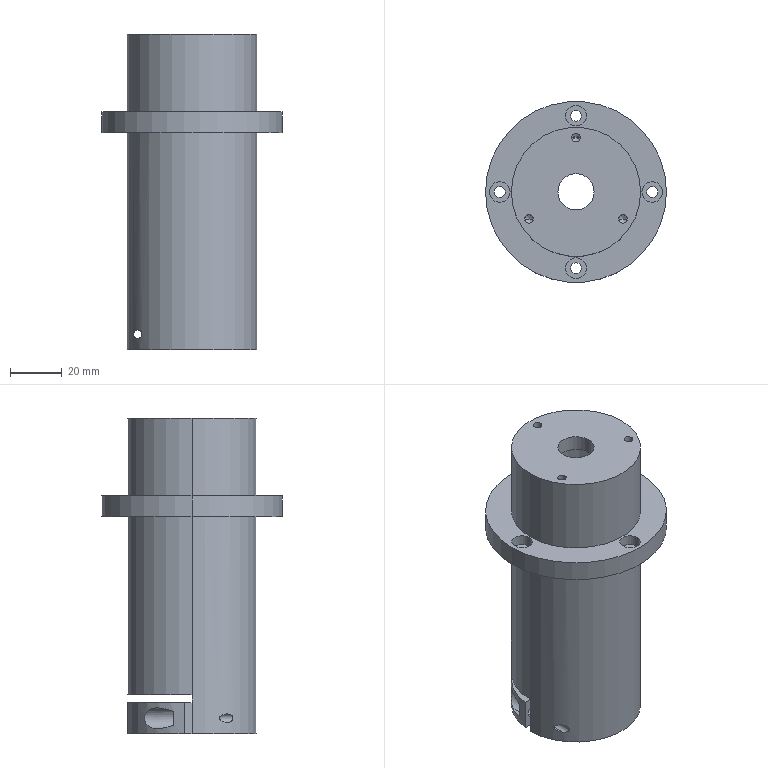Part | SolidWorks | features ICE 10, 3DProfileFeature 2, HoleWzd 2, Extrusion 1 | 1 solid | 62 faces | box 70 x 70 x 122 mm | volume 138507 mm3 | cylinder 41 | plane 15 | cone 6 | commonest cylinder face diameters 8 x11 3.3 x8 4.2 x8 50 x5 35 x3 4.5 x2